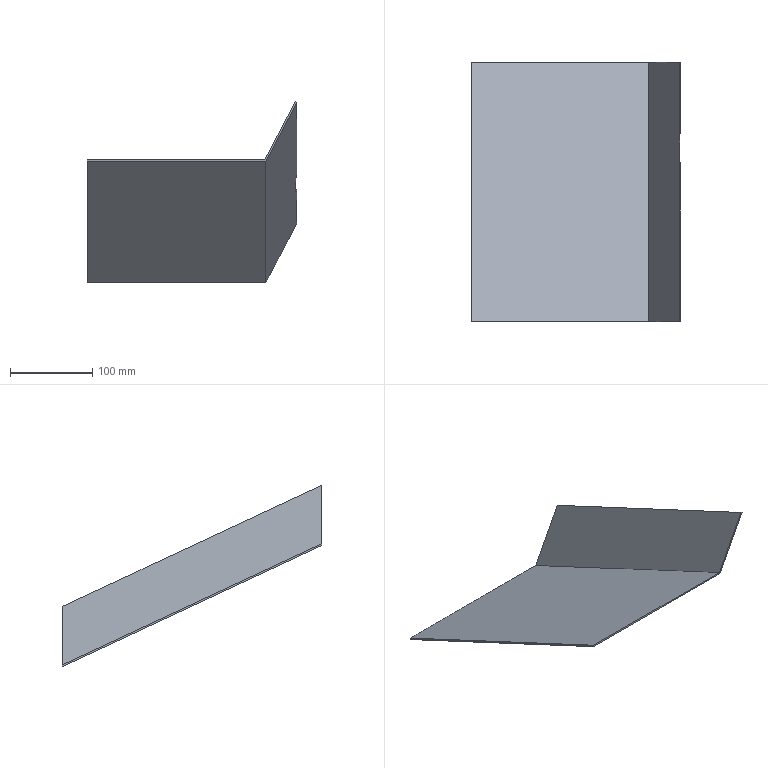Part | NX | features solid 2 | 1 solid | 10 faces | box 254.539 x 315 x 219.976 mm | volume 202205 mm3 | plane 9 | spline 1
STEP:
#1=CARTESIAN_POINT('',(-777.274,80.,-72.399));
#2=VERTEX_POINT('',#1);
#3=CARTESIAN_POINT('',(-775.461,80.,-73.348));
#4=VERTEX_POINT('',#3);
#5=CARTESIAN_POINT('',(-729.153,80.,-97.579));
#6=DIRECTION('',(0.886,0.,-0.4636));
#7=VECTOR('',#6,1000.);
#8=LINE('',#5,#7);
#9=EDGE_CURVE('',#2,#4,#8,.T.);
#10=ORIENTED_EDGE('',*,*,#9,.F.);
#11=CARTESIAN_POINT('',(-814.364,80.,-143.282));
#12=VERTEX_POINT('',#11);
#13=CARTESIAN_POINT('',(-854.375,80.,-219.747));
#14=DIRECTION('',(0.4636,0.,0.886));
#15=VECTOR('',#14,1000.);
#16=LINE('',#13,#15);
#17=EDGE_CURVE('',#12,#2,#16,.T.);
#18=ORIENTED_EDGE('',*,*,#17,.F.);
#19=CARTESIAN_POINT('',(-1030.,80.,-143.282));
#20=VERTEX_POINT('',#19);
#21=CARTESIAN_POINT('',(-930.,80.,-143.282));
#22=DIRECTION('',(1.,0.,0.));
#23=VECTOR('',#22,1000.);
#24=LINE('',#21,#23);
#25=EDGE_CURVE('',#20,#12,#24,.T.);
#26=ORIENTED_EDGE('',*,*,#25,.F.);
#27=CARTESIAN_POINT('',(-1030.,80.,-145.488));
#28=VERTEX_POINT('',#27);
#29=CARTESIAN_POINT('',(-1030.,80.,-150.));
#30=DIRECTION('',(0.,0.,1.));
#31=VECTOR('',#30,1000.);
#32=LINE('',#29,#31);
#33=EDGE_CURVE('',#28,#20,#32,.T.);
#34=ORIENTED_EDGE('',*,*,#33,.F.);
#35=CARTESIAN_POINT('',(-813.209,80.,-145.488));
#36=VERTEX_POINT('',#35);
#37=CARTESIAN_POINT('',(-930.,80.,-145.488));
#38=DIRECTION('',(1.,0.,0.));
#39=VECTOR('',#38,1000.);
#40=LINE('',#37,#39);
#41=EDGE_CURVE('',#28,#36,#40,.T.);
#42=ORIENTED_EDGE('',*,*,#41,.T.);
#43=CARTESIAN_POINT('',(-852.562,80.,-220.696));
#44=DIRECTION('',(0.4636,0.,0.886));
#45=VECTOR('',#44,1000.);
#46=LINE('',#43,#45);
#47=EDGE_CURVE('',#36,#4,#46,.T.);
#48=ORIENTED_EDGE('',*,*,#47,.T.);
#49=EDGE_LOOP('',(#10,#18,#26,#34,#42,#48));
#50=FACE_BOUND('',#49,.T.);
#51=CARTESIAN_POINT('',(-734.365,80.,-107.54));
#52=DIRECTION('',(0.,1.,0.));
#53=DIRECTION('',(-1.,0.,0.));
#54=AXIS2_PLACEMENT_3D('',#51,#52,#53);
#55=PLANE('',#54);
#56=ADVANCED_FACE('',(#50),#55,.F.);
#57=CARTESIAN_POINT('',(-777.274,395.,-219.286));
#58=VERTEX_POINT('',#57);
#59=CARTESIAN_POINT('',(-777.274,302.521,-176.162));
#60=VERTEX_POINT('',#59);
#61=CARTESIAN_POINT('',(-777.274,465.78,-252.291));
#62=DIRECTION('',(0.,-0.9063,0.4226));
#63=VECTOR('',#62,1000.);
#64=LINE('',#61,#63);
#65=EDGE_CURVE('',#58,#60,#64,.T.);
#66=ORIENTED_EDGE('',*,*,#65,.F.);
#67=CARTESIAN_POINT('',(-814.364,395.,-290.168));
#68=VERTEX_POINT('',#67);
#69=CARTESIAN_POINT('',(-794.036,395.,-251.32));
#70=DIRECTION('',(0.4636,0.,0.886));
#71=VECTOR('',#70,1000.);
#72=LINE('',#69,#71);
#73=EDGE_CURVE('',#68,#58,#72,.T.);
#74=ORIENTED_EDGE('',*,*,#73,.F.);
#75=CARTESIAN_POINT('',(-814.364,438.631,-310.514));
#76=DIRECTION('',(0.,-0.9063,0.4226));
#77=VECTOR('',#76,1000.);
#78=LINE('',#75,#77);
#79=EDGE_CURVE('',#68,#12,#78,.T.);
#80=ORIENTED_EDGE('',*,*,#79,.T.);
#81=ORIENTED_EDGE('',*,*,#17,.T.);
#82=CARTESIAN_POINT('',(-777.274,297.853,-173.985));
#83=VERTEX_POINT('',#82);
#84=CARTESIAN_POINT('',(-777.274,465.78,-252.291));
#85=DIRECTION('',(0.,-0.9063,0.4226));
#86=VECTOR('',#85,1000.);
#87=LINE('',#84,#86);
#88=EDGE_CURVE('',#83,#2,#87,.T.);
#89=ORIENTED_EDGE('',*,*,#88,.F.);
#90=CARTESIAN_POINT('',(-777.274,297.853,-173.985));
#91=CARTESIAN_POINT('',(-777.323,299.376,-174.789));
#92=CARTESIAN_POINT('',(-777.345,300.925,-175.555));
#93=CARTESIAN_POINT('',(-777.274,302.521,-176.162));
#94=B_SPLINE_CURVE_WITH_KNOTS('',3,(#90,#91,#92,#93),.UNSPECIFIED.,.F.,.F.,(4,4),(0.3237,0.3283),.UNSPECIFIED.);
#95=EDGE_CURVE('',#83,#60,#94,.T.);
#96=ORIENTED_EDGE('',*,*,#95,.T.);
#97=EDGE_LOOP('',(#66,#74,#80,#81,#89,#96));
#98=FACE_BOUND('',#97,.T.);
#99=CARTESIAN_POINT('',(-781.,463.053,-258.141));
#100=DIRECTION('',(0.866,-0.2113,-0.4532));
#101=DIRECTION('',(0.,-0.9063,0.4226));
#102=AXIS2_PLACEMENT_3D('',#99,#100,#101);
#103=PLANE('',#102);
#104=ADVANCED_FACE('',(#98),#103,.F.);
#105=CARTESIAN_POINT('',(-813.209,395.,-292.375));
#106=VERTEX_POINT('',#105);
#107=CARTESIAN_POINT('',(-775.461,395.,-220.235));
#108=VERTEX_POINT('',#107);
#109=CARTESIAN_POINT('',(-792.223,395.,-252.268));
#110=DIRECTION('',(0.4636,0.,0.886));
#111=VECTOR('',#110,1000.);
#112=LINE('',#109,#111);
#113=EDGE_CURVE('',#106,#108,#112,.T.);
#114=ORIENTED_EDGE('',*,*,#113,.T.);
#115=CARTESIAN_POINT('',(-775.461,311.039,-181.083));
#116=VERTEX_POINT('',#115);
#117=CARTESIAN_POINT('',(-775.461,465.417,-253.071));
#118=DIRECTION('',(0.,-0.9063,0.4226));
#119=VECTOR('',#118,1000.);
#120=LINE('',#117,#119);
#121=EDGE_CURVE('',#108,#116,#120,.T.);
#122=ORIENTED_EDGE('',*,*,#121,.T.);
#123=CARTESIAN_POINT('',(-775.461,268.117,-161.068));
#124=VERTEX_POINT('',#123);
#125=CARTESIAN_POINT('',(-775.461,268.117,-161.068));
#126=CARTESIAN_POINT('',(-775.834,269.591,-162.469));
#127=CARTESIAN_POINT('',(-776.525,272.654,-165.218));
#128=CARTESIAN_POINT('',(-777.077,277.727,-168.637));
#129=CARTESIAN_POINT('',(-777.023,283.295,-171.131));
#130=CARTESIAN_POINT('',(-776.974,288.864,-173.634));
#131=CARTESIAN_POINT('',(-777.108,294.276,-176.415));
#132=CARTESIAN_POINT('',(-777.383,299.569,-179.407));
#133=CARTESIAN_POINT('',(-777.27,304.257,-181.377));
#134=CARTESIAN_POINT('',(-776.563,308.299,-181.911));
#135=CARTESIAN_POINT('',(-775.877,310.206,-181.489));
#136=CARTESIAN_POINT('',(-775.461,311.039,-181.083));
#137=B_SPLINE_CURVE_WITH_KNOTS('',3,(#125,#126,#127,#128,#129,#130,#131,#132,#133,#134,#135,#136),.UNSPECIFIED.,.F.,.F.,(4,1,1,1,1,1,1,1,1,4),(0.2983,0.3039,0.3095,0.3151,0.3207,0.3263,0.3319,0.3375,0.3403,0.3431),.UNSPECIFIED.);
#138=EDGE_CURVE('',#124,#116,#137,.T.);
#139=ORIENTED_EDGE('',*,*,#138,.F.);
#140=CARTESIAN_POINT('',(-775.461,465.417,-253.071));
#141=DIRECTION('',(0.,-0.9063,0.4226));
#142=VECTOR('',#141,1000.);
#143=LINE('',#140,#142);
#144=EDGE_CURVE('',#124,#4,#143,.T.);
#145=ORIENTED_EDGE('',*,*,#144,.T.);
#146=ORIENTED_EDGE('',*,*,#47,.F.);
#147=CARTESIAN_POINT('',(-813.209,437.785,-312.326));
#148=DIRECTION('',(0.,-0.9063,0.4226));
#149=VECTOR('',#148,1000.);
#150=LINE('',#147,#149);
#151=EDGE_CURVE('',#106,#36,#150,.T.);
#152=ORIENTED_EDGE('',*,*,#151,.F.);
#153=EDGE_LOOP('',(#114,#122,#139,#145,#146,#152));
#154=FACE_BOUND('',#153,.T.);
#155=CARTESIAN_POINT('',(-779.268,462.63,-259.047));
#156=DIRECTION('',(0.866,-0.2113,-0.4532));
#157=DIRECTION('',(0.,-0.9063,0.4226));
#158=AXIS2_PLACEMENT_3D('',#155,#156,#157);
#159=PLANE('',#158);
#160=ADVANCED_FACE('',(#154),#159,.T.);
#161=ORIENTED_EDGE('',*,*,#73,.T.);
#162=CARTESIAN_POINT('',(-936.634,395.,-135.9));
#163=DIRECTION('',(0.886,0.,-0.4636));
#164=VECTOR('',#163,1000.);
#165=LINE('',#162,#164);
#166=EDGE_CURVE('',#58,#108,#165,.T.);
#167=ORIENTED_EDGE('',*,*,#166,.T.);
#168=ORIENTED_EDGE('',*,*,#113,.F.);
#169=CARTESIAN_POINT('',(-1030.,395.,-292.375));
#170=VERTEX_POINT('',#169);
#171=CARTESIAN_POINT('',(-930.,395.,-292.375));
#172=DIRECTION('',(1.,0.,0.));
#173=VECTOR('',#172,1000.);
#174=LINE('',#171,#173);
#175=EDGE_CURVE('',#170,#106,#174,.T.);
#176=ORIENTED_EDGE('',*,*,#175,.F.);
#177=CARTESIAN_POINT('',(-1030.,395.,-290.168));
#178=VERTEX_POINT('',#177);
#179=CARTESIAN_POINT('',(-1030.,395.,-150.));
#180=DIRECTION('',(0.,0.,1.));
#181=VECTOR('',#180,1000.);
#182=LINE('',#179,#181);
#183=EDGE_CURVE('',#170,#178,#182,.T.);
#184=ORIENTED_EDGE('',*,*,#183,.T.);
#185=CARTESIAN_POINT('',(-930.,395.,-290.168));
#186=DIRECTION('',(1.,0.,0.));
#187=VECTOR('',#186,1000.);
#188=LINE('',#185,#187);
#189=EDGE_CURVE('',#178,#68,#188,.T.);
#190=ORIENTED_EDGE('',*,*,#189,.T.);
#191=EDGE_LOOP('',(#161,#167,#168,#176,#184,#190));
#192=FACE_BOUND('',#191,.T.);
#193=CARTESIAN_POINT('',(-910.,395.,-85.));
#194=DIRECTION('',(0.,1.,0.));
#195=DIRECTION('',(0.,0.,-1.));
#196=AXIS2_PLACEMENT_3D('',#193,#194,#195);
#197=PLANE('',#196);
#198=ADVANCED_FACE('',(#192),#197,.T.);
#199=CARTESIAN_POINT('',(-775.461,268.117,-161.068));
#200=CARTESIAN_POINT('',(-776.089,270.598,-161.896));
#201=CARTESIAN_POINT('',(-777.068,275.556,-163.696));
#202=CARTESIAN_POINT('',(-777.037,282.974,-167.171));
#203=CARTESIAN_POINT('',(-776.947,290.38,-170.672));
#204=CARTESIAN_POINT('',(-777.194,295.368,-172.868));
#205=CARTESIAN_POINT('',(-777.274,297.853,-173.985));
#206=B_SPLINE_CURVE_WITH_KNOTS('',3,(#199,#200,#201,#202,#203,#204,#205),.UNSPECIFIED.,.F.,.F.,(4,1,1,1,4),(0.2149,0.2229,0.2309,0.2389,0.247),.UNSPECIFIED.);
#207=EDGE_CURVE('',#124,#83,#206,.T.);
#208=ORIENTED_EDGE('',*,*,#207,.F.);
#209=ORIENTED_EDGE('',*,*,#138,.T.);
#210=CARTESIAN_POINT('',(-777.274,302.521,-176.162));
#211=CARTESIAN_POINT('',(-777.14,305.516,-177.629));
#212=CARTESIAN_POINT('',(-776.725,308.507,-179.241));
#213=CARTESIAN_POINT('',(-775.461,311.039,-181.083));
#214=B_SPLINE_CURVE_WITH_KNOTS('',3,(#210,#211,#212,#213),.UNSPECIFIED.,.F.,.F.,(4,4),(0.252,0.2619),.UNSPECIFIED.);
#215=EDGE_CURVE('',#60,#116,#214,.T.);
#216=ORIENTED_EDGE('',*,*,#215,.F.);
#217=ORIENTED_EDGE('',*,*,#95,.F.);
#218=EDGE_LOOP('',(#208,#209,#216,#217));
#219=FACE_BOUND('',#218,.T.);
#220=CARTESIAN_POINT('',(-775.396,267.865,-160.944));
#221=CARTESIAN_POINT('',(-775.396,267.865,-181.898));
#222=CARTESIAN_POINT('',(-775.851,269.635,-160.944));
#223=CARTESIAN_POINT('',(-775.851,269.635,-181.898));
#224=CARTESIAN_POINT('',(-776.647,273.211,-160.944));
#225=CARTESIAN_POINT('',(-776.647,273.211,-181.898));
#226=CARTESIAN_POINT('',(-777.1,278.665,-160.944));
#227=CARTESIAN_POINT('',(-777.1,278.665,-181.898));
#228=CARTESIAN_POINT('',(-777.001,284.157,-160.944));
#229=CARTESIAN_POINT('',(-777.001,284.157,-181.898));
#230=CARTESIAN_POINT('',(-776.981,289.638,-160.944));
#231=CARTESIAN_POINT('',(-776.981,289.638,-181.898));
#232=CARTESIAN_POINT('',(-777.152,295.115,-160.944));
#233=CARTESIAN_POINT('',(-777.152,295.115,-181.898));
#234=CARTESIAN_POINT('',(-777.412,300.591,-160.944));
#235=CARTESIAN_POINT('',(-777.412,300.591,-181.898));
#236=CARTESIAN_POINT('',(-777.112,306.068,-160.944));
#237=CARTESIAN_POINT('',(-777.112,306.068,-181.898));
#238=CARTESIAN_POINT('',(-776.202,309.64,-160.944));
#239=CARTESIAN_POINT('',(-776.202,309.64,-181.898));
#240=CARTESIAN_POINT('',(-775.341,311.272,-160.944));
#241=CARTESIAN_POINT('',(-775.341,311.272,-181.898));
#242=B_SPLINE_SURFACE_WITH_KNOTS('',3,1,((#220,#221),(#222,#223),(#224,#225),(#226,#227),(#228,#229),(#230,#231),(#232,#233),(#234,#235),(#236,#237),(#238,#239),(#240,#241)),.SURF_OF_LINEAR_EXTRUSION.,.F.,.F.,.F.,(4,1,1,1,1,1,1,1,4),(2,2),(0.5139,0.5151,0.5163,0.5175,0.5187,0.5199,0.5211,0.5223,0.5235),(0.,1.),.UNSPECIFIED.);
#243=ADVANCED_FACE('',(#219),#242,.F.);
#244=ORIENTED_EDGE('',*,*,#79,.F.);
#245=ORIENTED_EDGE('',*,*,#189,.F.);
#246=CARTESIAN_POINT('',(-1030.,438.631,-310.514));
#247=DIRECTION('',(0.,-0.9063,0.4226));
#248=VECTOR('',#247,1000.);
#249=LINE('',#246,#248);
#250=EDGE_CURVE('',#178,#20,#249,.T.);
#251=ORIENTED_EDGE('',*,*,#250,.T.);
#252=ORIENTED_EDGE('',*,*,#25,.T.);
#253=EDGE_LOOP('',(#244,#245,#251,#252));
#254=FACE_BOUND('',#253,.T.);
#255=CARTESIAN_POINT('',(-930.,438.631,-310.514));
#256=DIRECTION('',(0.,-0.4226,-0.9063));
#257=DIRECTION('',(-1.,0.,0.));
#258=AXIS2_PLACEMENT_3D('',#255,#256,#257);
#259=PLANE('',#258);
#260=ADVANCED_FACE('',(#254),#259,.F.);
#261=ORIENTED_EDGE('',*,*,#250,.F.);
#262=ORIENTED_EDGE('',*,*,#183,.F.);
#263=CARTESIAN_POINT('',(-1030.,437.785,-312.326));
#264=DIRECTION('',(0.,-0.9063,0.4226));
#265=VECTOR('',#264,1000.);
#266=LINE('',#263,#265);
#267=EDGE_CURVE('',#170,#28,#266,.T.);
#268=ORIENTED_EDGE('',*,*,#267,.T.);
#269=ORIENTED_EDGE('',*,*,#33,.T.);
#270=EDGE_LOOP('',(#261,#262,#268,#269));
#271=FACE_BOUND('',#270,.T.);
#272=CARTESIAN_POINT('',(-1030.,400.,-150.));
#273=DIRECTION('',(1.,0.,0.));
#274=DIRECTION('',(0.,0.,-1.));
#275=AXIS2_PLACEMENT_3D('',#272,#273,#274);
#276=PLANE('',#275);
#277=ADVANCED_FACE('',(#271),#276,.F.);
#278=ORIENTED_EDGE('',*,*,#175,.T.);
#279=ORIENTED_EDGE('',*,*,#151,.T.);
#280=ORIENTED_EDGE('',*,*,#41,.F.);
#281=ORIENTED_EDGE('',*,*,#267,.F.);
#282=EDGE_LOOP('',(#278,#279,#280,#281));
#283=FACE_BOUND('',#282,.T.);
#284=CARTESIAN_POINT('',(-930.,437.785,-312.326));
#285=DIRECTION('',(0.,-0.4226,-0.9063));
#286=DIRECTION('',(-1.,0.,0.));
#287=AXIS2_PLACEMENT_3D('',#284,#285,#286);
#288=PLANE('',#287);
#289=ADVANCED_FACE('',(#283),#288,.T.);
#290=ORIENTED_EDGE('',*,*,#166,.F.);
#291=ORIENTED_EDGE('',*,*,#65,.T.);
#292=ORIENTED_EDGE('',*,*,#215,.T.);
#293=ORIENTED_EDGE('',*,*,#121,.F.);
#294=EDGE_LOOP('',(#290,#291,#292,#293));
#295=FACE_BOUND('',#294,.T.);
#296=CARTESIAN_POINT('',(-777.274,395.,-219.286));
#297=DIRECTION('',(0.4285,0.3819,0.8189));
#298=DIRECTION('',(0.886,0.,-0.4636));
#299=AXIS2_PLACEMENT_3D('',#296,#297,#298);
#300=PLANE('',#299);
#301=ADVANCED_FACE('',(#295),#300,.T.);
#302=ORIENTED_EDGE('',*,*,#88,.T.);
#303=ORIENTED_EDGE('',*,*,#9,.T.);
#304=ORIENTED_EDGE('',*,*,#144,.F.);
#305=ORIENTED_EDGE('',*,*,#207,.T.);
#306=EDGE_LOOP('',(#302,#303,#304,#305));
#307=FACE_BOUND('',#306,.T.);
#308=CARTESIAN_POINT('',(-777.274,395.,-219.286));
#309=DIRECTION('',(0.4285,0.3819,0.8189));
#310=DIRECTION('',(0.886,0.,-0.4636));
#311=AXIS2_PLACEMENT_3D('',#308,#309,#310);
#312=PLANE('',#311);
#313=ADVANCED_FACE('',(#307),#312,.T.);
#314=CLOSED_SHELL('',(#56,#104,#160,#198,#243,#260,#277,#289,#301,#313));
#315=MANIFOLD_SOLID_BREP('',#314);
#316=(LENGTH_UNIT()NAMED_UNIT(*)SI_UNIT(.MILLI.,.METRE.));
#317=UNCERTAINTY_MEASURE_WITH_UNIT(LENGTH_MEASURE(0.0508),#316,'','');
#318=(NAMED_UNIT(*)PLANE_ANGLE_UNIT()SI_UNIT($,.RADIAN.));
#319=(NAMED_UNIT(*)SI_UNIT($,.STERADIAN.)SOLID_ANGLE_UNIT());
#320=(GEOMETRIC_REPRESENTATION_CONTEXT(3)GLOBAL_UNCERTAINTY_ASSIGNED_CONTEXT((#317))GLOBAL_UNIT_ASSIGNED_CONTEXT((#316,#318,#319))REPRESENTATION_CONTEXT('',''));
#321=ADVANCED_BREP_SHAPE_REPRESENTATION('',(#315),#320);